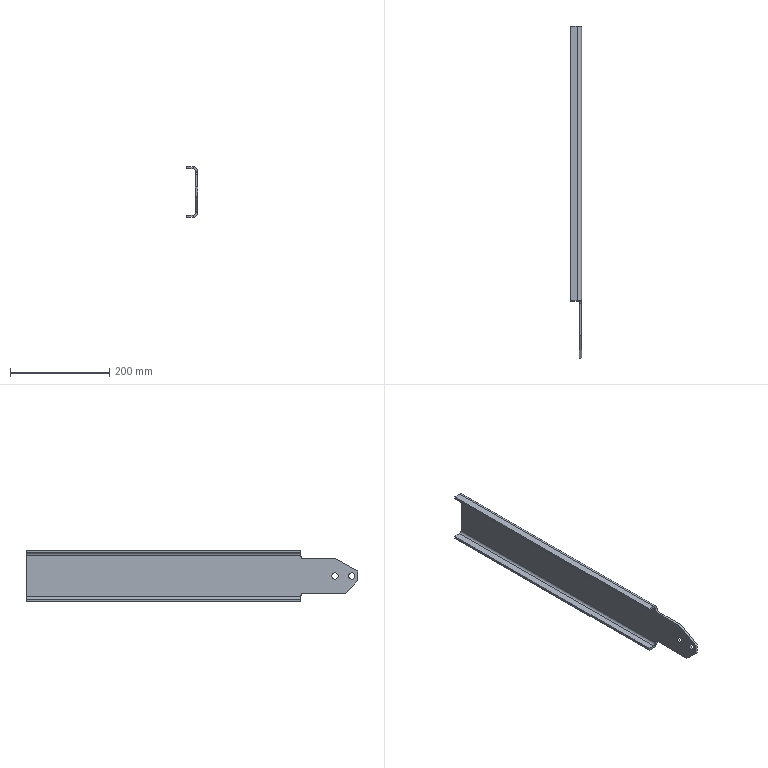Part | SolidWorks | features ICE 2, FlatPattern 1, SMBaseFlange 1, SheetMetal 1 | 1 solid | 41 faces | box 22.5 x 670 x 102.2 mm | volume 361914 mm3 | plane 26 | cylinder 15 | commonest cylinder face diameters 26.5 x5 12.5 x4 9 x2 10 x2 18 x2
STEP:
#1=CARTESIAN_POINT('',(22.499,46.5,59.85));
#2=VERTEX_POINT('',#1);
#3=CARTESIAN_POINT('',(22.499,46.5,33.35));
#4=VERTEX_POINT('',#3);
#5=CARTESIAN_POINT('',(22.499,46.5,46.6));
#6=DIRECTION('',(1.,0.,0.));
#7=DIRECTION('',(0.,0.,-1.));
#8=AXIS2_PLACEMENT_3D('',#5,#6,#7);
#9=CIRCLE('',#8,13.25);
#10=EDGE_CURVE('',#2,#4,#9,.T.);
#11=ORIENTED_EDGE('',*,*,#10,.F.);
#12=CARTESIAN_POINT('',(22.5,46.5,59.85));
#13=VERTEX_POINT('',#12);
#14=CARTESIAN_POINT('',(22.499,46.5,59.85));
#15=DIRECTION('',(1.,0.,0.));
#16=VECTOR('',#15,1000.);
#17=LINE('',#14,#16);
#18=EDGE_CURVE('',#2,#13,#17,.T.);
#19=ORIENTED_EDGE('',*,*,#18,.T.);
#20=CARTESIAN_POINT('',(22.5,46.5,33.35));
#21=VERTEX_POINT('',#20);
#22=CARTESIAN_POINT('',(22.5,46.5,46.6));
#23=DIRECTION('',(1.,0.,0.));
#24=DIRECTION('',(0.,0.,-1.));
#25=AXIS2_PLACEMENT_3D('',#22,#23,#24);
#26=CIRCLE('',#25,13.25);
#27=EDGE_CURVE('',#13,#21,#26,.T.);
#28=ORIENTED_EDGE('',*,*,#27,.T.);
#29=CARTESIAN_POINT('',(22.499,46.5,33.35));
#30=DIRECTION('',(1.,0.,0.));
#31=VECTOR('',#30,1000.);
#32=LINE('',#29,#31);
#33=EDGE_CURVE('',#4,#21,#32,.T.);
#34=ORIENTED_EDGE('',*,*,#33,.F.);
#35=EDGE_LOOP('',(#11,#19,#28,#34));
#36=FACE_OUTER_BOUND('',#35,.T.);
#37=CARTESIAN_POINT('',(22.499,46.5,46.6));
#38=DIRECTION('',(1.,0.,0.));
#39=DIRECTION('',(0.,0.,-1.));
#40=AXIS2_PLACEMENT_3D('',#37,#38,#39);
#41=CYLINDRICAL_SURFACE('',#40,13.25);
#42=ADVANCED_FACE('',(#36),#41,.F.);
#43=CARTESIAN_POINT('',(22.499,12.5,59.85));
#44=VERTEX_POINT('',#43);
#45=CARTESIAN_POINT('',(22.499,0.,50.995));
#46=VERTEX_POINT('',#45);
#47=CARTESIAN_POINT('',(22.499,12.5,46.6));
#48=DIRECTION('',(1.,0.,0.));
#49=DIRECTION('',(0.,0.,-1.));
#50=AXIS2_PLACEMENT_3D('',#47,#48,#49);
#51=CIRCLE('',#50,13.25);
#52=EDGE_CURVE('',#44,#46,#51,.T.);
#53=ORIENTED_EDGE('',*,*,#52,.F.);
#54=CARTESIAN_POINT('',(22.5,12.5,59.85));
#55=VERTEX_POINT('',#54);
#56=CARTESIAN_POINT('',(22.499,12.5,59.85));
#57=DIRECTION('',(1.,0.,0.));
#58=VECTOR('',#57,1000.);
#59=LINE('',#56,#58);
#60=EDGE_CURVE('',#44,#55,#59,.T.);
#61=ORIENTED_EDGE('',*,*,#60,.T.);
#62=CARTESIAN_POINT('',(22.5,0.,50.995));
#63=VERTEX_POINT('',#62);
#64=CARTESIAN_POINT('',(22.5,12.5,46.6));
#65=DIRECTION('',(1.,0.,0.));
#66=DIRECTION('',(0.,0.,-1.));
#67=AXIS2_PLACEMENT_3D('',#64,#65,#66);
#68=CIRCLE('',#67,13.25);
#69=EDGE_CURVE('',#55,#63,#68,.T.);
#70=ORIENTED_EDGE('',*,*,#69,.T.);
#71=CARTESIAN_POINT('',(22.499,0.,50.995));
#72=DIRECTION('',(-1.,0.,0.));
#73=VECTOR('',#72,1000.);
#74=LINE('',#71,#73);
#75=EDGE_CURVE('',#63,#46,#74,.T.);
#76=ORIENTED_EDGE('',*,*,#75,.T.);
#77=EDGE_LOOP('',(#53,#61,#70,#76));
#78=FACE_OUTER_BOUND('',#77,.T.);
#79=CARTESIAN_POINT('',(22.499,12.5,46.6));
#80=DIRECTION('',(1.,0.,0.));
#81=DIRECTION('',(0.,0.,-1.));
#82=AXIS2_PLACEMENT_3D('',#79,#80,#81);
#83=CYLINDRICAL_SURFACE('',#82,13.25);
#84=ADVANCED_FACE('',(#78),#83,.F.);
#85=ORIENTED_EDGE('',*,*,#60,.F.);
#86=CARTESIAN_POINT('',(22.499,12.5,33.35));
#87=VERTEX_POINT('',#86);
#88=CARTESIAN_POINT('',(22.499,12.5,46.6));
#89=DIRECTION('',(1.,0.,0.));
#90=DIRECTION('',(0.,0.,-1.));
#91=AXIS2_PLACEMENT_3D('',#88,#89,#90);
#92=CIRCLE('',#91,13.25);
#93=EDGE_CURVE('',#87,#44,#92,.T.);
#94=ORIENTED_EDGE('',*,*,#93,.F.);
#95=CARTESIAN_POINT('',(22.5,12.5,33.35));
#96=VERTEX_POINT('',#95);
#97=CARTESIAN_POINT('',(22.499,12.5,33.35));
#98=DIRECTION('',(1.,0.,0.));
#99=VECTOR('',#98,1000.);
#100=LINE('',#97,#99);
#101=EDGE_CURVE('',#87,#96,#100,.T.);
#102=ORIENTED_EDGE('',*,*,#101,.T.);
#103=CARTESIAN_POINT('',(22.5,12.5,46.6));
#104=DIRECTION('',(1.,0.,0.));
#105=DIRECTION('',(0.,0.,-1.));
#106=AXIS2_PLACEMENT_3D('',#103,#104,#105);
#107=CIRCLE('',#106,13.25);
#108=EDGE_CURVE('',#96,#55,#107,.T.);
#109=ORIENTED_EDGE('',*,*,#108,.T.);
#110=EDGE_LOOP('',(#85,#94,#102,#109));
#111=FACE_OUTER_BOUND('',#110,.T.);
#112=CARTESIAN_POINT('',(22.499,12.5,46.6));
#113=DIRECTION('',(1.,0.,0.));
#114=DIRECTION('',(0.,0.,-1.));
#115=AXIS2_PLACEMENT_3D('',#112,#113,#114);
#116=CYLINDRICAL_SURFACE('',#115,13.25);
#117=ADVANCED_FACE('',(#111),#116,.F.);
#118=CARTESIAN_POINT('',(18.,12.5,52.85));
#119=VERTEX_POINT('',#118);
#120=CARTESIAN_POINT('',(18.,12.5,40.35));
#121=VERTEX_POINT('',#120);
#122=CARTESIAN_POINT('',(18.,12.5,46.6));
#123=DIRECTION('',(1.,0.,0.));
#124=DIRECTION('',(0.,0.,-1.));
#125=AXIS2_PLACEMENT_3D('',#122,#123,#124);
#126=CIRCLE('',#125,6.25);
#127=EDGE_CURVE('',#119,#121,#126,.T.);
#128=ORIENTED_EDGE('',*,*,#127,.F.);
#129=CARTESIAN_POINT('',(22.499,12.5,52.85));
#130=VERTEX_POINT('',#129);
#131=CARTESIAN_POINT('',(22.5,12.5,52.85));
#132=DIRECTION('',(1.,0.,0.));
#133=VECTOR('',#132,1000.);
#134=LINE('',#131,#133);
#135=EDGE_CURVE('',#119,#130,#134,.T.);
#136=ORIENTED_EDGE('',*,*,#135,.T.);
#137=CARTESIAN_POINT('',(22.499,12.5,40.35));
#138=VERTEX_POINT('',#137);
#139=CARTESIAN_POINT('',(22.499,12.5,46.6));
#140=DIRECTION('',(1.,0.,0.));
#141=DIRECTION('',(0.,0.,-1.));
#142=AXIS2_PLACEMENT_3D('',#139,#140,#141);
#143=CIRCLE('',#142,6.25);
#144=EDGE_CURVE('',#130,#138,#143,.T.);
#145=ORIENTED_EDGE('',*,*,#144,.T.);
#146=CARTESIAN_POINT('',(22.5,12.5,40.35));
#147=DIRECTION('',(1.,0.,0.));
#148=VECTOR('',#147,1000.);
#149=LINE('',#146,#148);
#150=EDGE_CURVE('',#121,#138,#149,.T.);
#151=ORIENTED_EDGE('',*,*,#150,.F.);
#152=EDGE_LOOP('',(#128,#136,#145,#151));
#153=FACE_OUTER_BOUND('',#152,.T.);
#154=CARTESIAN_POINT('',(22.5,12.5,46.6));
#155=DIRECTION('',(1.,0.,0.));
#156=DIRECTION('',(0.,0.,-1.));
#157=AXIS2_PLACEMENT_3D('',#154,#155,#156);
#158=CYLINDRICAL_SURFACE('',#157,6.25);
#159=ADVANCED_FACE('',(#153),#158,.F.);
#160=CARTESIAN_POINT('',(18.,46.5,52.85));
#161=VERTEX_POINT('',#160);
#162=CARTESIAN_POINT('',(18.,46.5,40.35));
#163=VERTEX_POINT('',#162);
#164=CARTESIAN_POINT('',(18.,46.5,46.6));
#165=DIRECTION('',(1.,0.,0.));
#166=DIRECTION('',(0.,0.,-1.));
#167=AXIS2_PLACEMENT_3D('',#164,#165,#166);
#168=CIRCLE('',#167,6.25);
#169=EDGE_CURVE('',#161,#163,#168,.T.);
#170=ORIENTED_EDGE('',*,*,#169,.F.);
#171=CARTESIAN_POINT('',(22.499,46.5,52.85));
#172=VERTEX_POINT('',#171);
#173=CARTESIAN_POINT('',(22.5,46.5,52.85));
#174=DIRECTION('',(1.,0.,0.));
#175=VECTOR('',#174,1000.);
#176=LINE('',#173,#175);
#177=EDGE_CURVE('',#161,#172,#176,.T.);
#178=ORIENTED_EDGE('',*,*,#177,.T.);
#179=CARTESIAN_POINT('',(22.499,46.5,40.35));
#180=VERTEX_POINT('',#179);
#181=CARTESIAN_POINT('',(22.499,46.5,46.6));
#182=DIRECTION('',(1.,0.,0.));
#183=DIRECTION('',(0.,0.,-1.));
#184=AXIS2_PLACEMENT_3D('',#181,#182,#183);
#185=CIRCLE('',#184,6.25);
#186=EDGE_CURVE('',#172,#180,#185,.T.);
#187=ORIENTED_EDGE('',*,*,#186,.T.);
#188=CARTESIAN_POINT('',(22.5,46.5,40.35));
#189=DIRECTION('',(1.,0.,0.));
#190=VECTOR('',#189,1000.);
#191=LINE('',#188,#190);
#192=EDGE_CURVE('',#163,#180,#191,.T.);
#193=ORIENTED_EDGE('',*,*,#192,.F.);
#194=EDGE_LOOP('',(#170,#178,#187,#193));
#195=FACE_OUTER_BOUND('',#194,.T.);
#196=CARTESIAN_POINT('',(22.5,46.5,46.6));
#197=DIRECTION('',(1.,0.,0.));
#198=DIRECTION('',(0.,0.,-1.));
#199=AXIS2_PLACEMENT_3D('',#196,#197,#198);
#200=CYLINDRICAL_SURFACE('',#199,6.25);
#201=ADVANCED_FACE('',(#195),#200,.F.);
#202=ORIENTED_EDGE('',*,*,#177,.F.);
#203=CARTESIAN_POINT('',(18.,46.5,46.6));
#204=DIRECTION('',(1.,0.,0.));
#205=DIRECTION('',(0.,0.,-1.));
#206=AXIS2_PLACEMENT_3D('',#203,#204,#205);
#207=CIRCLE('',#206,6.25);
#208=EDGE_CURVE('',#163,#161,#207,.T.);
#209=ORIENTED_EDGE('',*,*,#208,.F.);
#210=ORIENTED_EDGE('',*,*,#192,.T.);
#211=CARTESIAN_POINT('',(22.499,46.5,46.6));
#212=DIRECTION('',(1.,0.,0.));
#213=DIRECTION('',(0.,0.,-1.));
#214=AXIS2_PLACEMENT_3D('',#211,#212,#213);
#215=CIRCLE('',#214,6.25);
#216=EDGE_CURVE('',#180,#172,#215,.T.);
#217=ORIENTED_EDGE('',*,*,#216,.T.);
#218=EDGE_LOOP('',(#202,#209,#210,#217));
#219=FACE_OUTER_BOUND('',#218,.T.);
#220=CARTESIAN_POINT('',(22.5,46.5,46.6));
#221=DIRECTION('',(1.,0.,0.));
#222=DIRECTION('',(0.,0.,-1.));
#223=AXIS2_PLACEMENT_3D('',#220,#221,#222);
#224=CYLINDRICAL_SURFACE('',#223,6.25);
#225=ADVANCED_FACE('',(#219),#224,.F.);
#226=ORIENTED_EDGE('',*,*,#135,.F.);
#227=CARTESIAN_POINT('',(18.,12.5,46.6));
#228=DIRECTION('',(1.,0.,0.));
#229=DIRECTION('',(0.,0.,-1.));
#230=AXIS2_PLACEMENT_3D('',#227,#228,#229);
#231=CIRCLE('',#230,6.25);
#232=EDGE_CURVE('',#121,#119,#231,.T.);
#233=ORIENTED_EDGE('',*,*,#232,.F.);
#234=ORIENTED_EDGE('',*,*,#150,.T.);
#235=CARTESIAN_POINT('',(22.499,12.5,46.6));
#236=DIRECTION('',(1.,0.,0.));
#237=DIRECTION('',(0.,0.,-1.));
#238=AXIS2_PLACEMENT_3D('',#235,#236,#237);
#239=CIRCLE('',#238,6.25);
#240=EDGE_CURVE('',#138,#130,#239,.T.);
#241=ORIENTED_EDGE('',*,*,#240,.T.);
#242=EDGE_LOOP('',(#226,#233,#234,#241));
#243=FACE_OUTER_BOUND('',#242,.T.);
#244=CARTESIAN_POINT('',(22.5,12.5,46.6));
#245=DIRECTION('',(1.,0.,0.));
#246=DIRECTION('',(0.,0.,-1.));
#247=AXIS2_PLACEMENT_3D('',#244,#245,#246);
#248=CYLINDRICAL_SURFACE('',#247,6.25);
#249=ADVANCED_FACE('',(#243),#248,.F.);
#250=CARTESIAN_POINT('',(22.499,0.,42.205));
#251=VERTEX_POINT('',#250);
#252=CARTESIAN_POINT('',(22.5,0.,42.205));
#253=VERTEX_POINT('',#252);
#254=CARTESIAN_POINT('',(22.499,0.,42.205));
#255=DIRECTION('',(1.,0.,0.));
#256=VECTOR('',#255,1000.);
#257=LINE('',#254,#256);
#258=EDGE_CURVE('',#251,#253,#257,.T.);
#259=ORIENTED_EDGE('',*,*,#258,.F.);
#260=CARTESIAN_POINT('',(22.499,0.,-4.5));
#261=DIRECTION('',(0.,0.,1.));
#262=VECTOR('',#261,1000.);
#263=LINE('',#260,#262);
#264=EDGE_CURVE('',#251,#46,#263,.T.);
#265=ORIENTED_EDGE('',*,*,#264,.T.);
#266=ORIENTED_EDGE('',*,*,#75,.F.);
#267=CARTESIAN_POINT('',(22.5,0.,56.7));
#268=VERTEX_POINT('',#267);
#269=CARTESIAN_POINT('',(22.5,0.,0.));
#270=DIRECTION('',(0.,0.,1.));
#271=VECTOR('',#270,1000.);
#272=LINE('',#269,#271);
#273=EDGE_CURVE('',#63,#268,#272,.T.);
#274=ORIENTED_EDGE('',*,*,#273,.T.);
#275=CARTESIAN_POINT('',(18.,0.,56.7));
#276=VERTEX_POINT('',#275);
#277=CARTESIAN_POINT('',(22.5,0.,56.7));
#278=DIRECTION('',(-1.,0.,0.));
#279=VECTOR('',#278,1000.);
#280=LINE('',#277,#279);
#281=EDGE_CURVE('',#268,#276,#280,.T.);
#282=ORIENTED_EDGE('',*,*,#281,.T.);
#283=CARTESIAN_POINT('',(18.,0.,36.7));
#284=VERTEX_POINT('',#283);
#285=CARTESIAN_POINT('',(18.,0.,0.));
#286=DIRECTION('',(0.,0.,1.));
#287=VECTOR('',#286,1000.);
#288=LINE('',#285,#287);
#289=EDGE_CURVE('',#284,#276,#288,.T.);
#290=ORIENTED_EDGE('',*,*,#289,.F.);
#291=CARTESIAN_POINT('',(22.5,0.,36.7));
#292=VERTEX_POINT('',#291);
#293=CARTESIAN_POINT('',(22.5,0.,36.7));
#294=DIRECTION('',(-1.,0.,0.));
#295=VECTOR('',#294,1000.);
#296=LINE('',#293,#295);
#297=EDGE_CURVE('',#292,#284,#296,.T.);
#298=ORIENTED_EDGE('',*,*,#297,.F.);
#299=CARTESIAN_POINT('',(22.5,0.,0.));
#300=DIRECTION('',(0.,0.,1.));
#301=VECTOR('',#300,1000.);
#302=LINE('',#299,#301);
#303=EDGE_CURVE('',#292,#253,#302,.T.);
#304=ORIENTED_EDGE('',*,*,#303,.T.);
#305=EDGE_LOOP('',(#259,#265,#266,#274,#282,#290,#298,#304));
#306=FACE_OUTER_BOUND('',#305,.T.);
#307=CARTESIAN_POINT('',(13.5,0.,-4.5));
#308=DIRECTION('',(0.,-1.,0.));
#309=DIRECTION('',(0.,0.,-1.));
#310=AXIS2_PLACEMENT_3D('',#307,#308,#309);
#311=PLANE('',#310);
#312=ADVANCED_FACE('',(#306),#311,.T.);
#313=CARTESIAN_POINT('',(0.,115.,93.2));
#314=VERTEX_POINT('',#313);
#315=CARTESIAN_POINT('',(13.5,115.,93.2));
#316=VERTEX_POINT('',#315);
#317=CARTESIAN_POINT('',(18.,115.,93.2));
#318=DIRECTION('',(1.,0.,0.));
#319=VECTOR('',#318,1000.);
#320=LINE('',#317,#319);
#321=EDGE_CURVE('',#314,#316,#320,.T.);
#322=ORIENTED_EDGE('',*,*,#321,.F.);
#323=CARTESIAN_POINT('',(0.,670.,93.2));
#324=VERTEX_POINT('',#323);
#325=CARTESIAN_POINT('',(0.,670.,93.2));
#326=DIRECTION('',(0.,-1.,0.));
#327=VECTOR('',#326,1000.);
#328=LINE('',#325,#327);
#329=EDGE_CURVE('',#324,#314,#328,.T.);
#330=ORIENTED_EDGE('',*,*,#329,.F.);
#331=CARTESIAN_POINT('',(13.5,670.,93.2));
#332=VERTEX_POINT('',#331);
#333=CARTESIAN_POINT('',(18.,670.,93.2));
#334=DIRECTION('',(-1.,0.,0.));
#335=VECTOR('',#334,1000.);
#336=LINE('',#333,#335);
#337=EDGE_CURVE('',#332,#324,#336,.T.);
#338=ORIENTED_EDGE('',*,*,#337,.F.);
#339=CARTESIAN_POINT('',(13.5,670.,93.2));
#340=DIRECTION('',(0.,-1.,0.));
#341=VECTOR('',#340,1000.);
#342=LINE('',#339,#341);
#343=EDGE_CURVE('',#332,#316,#342,.T.);
#344=ORIENTED_EDGE('',*,*,#343,.T.);
#345=EDGE_LOOP('',(#322,#330,#338,#344));
#346=FACE_OUTER_BOUND('',#345,.T.);
#347=CARTESIAN_POINT('',(18.,670.,93.2));
#348=DIRECTION('',(0.,0.,1.));
#349=DIRECTION('',(1.,0.,0.));
#350=AXIS2_PLACEMENT_3D('',#347,#348,#349);
#351=PLANE('',#350);
#352=ADVANCED_FACE('',(#346),#351,.F.);
#353=ORIENTED_EDGE('',*,*,#329,.T.);
#354=CARTESIAN_POINT('',(0.,115.,97.7));
#355=VERTEX_POINT('',#354);
#356=CARTESIAN_POINT('',(0.,115.,97.7));
#357=DIRECTION('',(0.,0.,-1.));
#358=VECTOR('',#357,1000.);
#359=LINE('',#356,#358);
#360=EDGE_CURVE('',#355,#314,#359,.T.);
#361=ORIENTED_EDGE('',*,*,#360,.F.);
#362=CARTESIAN_POINT('',(0.,670.,97.7));
#363=VERTEX_POINT('',#362);
#364=CARTESIAN_POINT('',(0.,670.,97.7));
#365=DIRECTION('',(0.,-1.,0.));
#366=VECTOR('',#365,1000.);
#367=LINE('',#364,#366);
#368=EDGE_CURVE('',#363,#355,#367,.T.);
#369=ORIENTED_EDGE('',*,*,#368,.F.);
#370=CARTESIAN_POINT('',(0.,670.,97.7));
#371=DIRECTION('',(0.,0.,-1.));
#372=VECTOR('',#371,1000.);
#373=LINE('',#370,#372);
#374=EDGE_CURVE('',#363,#324,#373,.T.);
#375=ORIENTED_EDGE('',*,*,#374,.T.);
#376=EDGE_LOOP('',(#353,#361,#369,#375));
#377=FACE_OUTER_BOUND('',#376,.T.);
#378=CARTESIAN_POINT('',(0.,670.,97.7));
#379=DIRECTION('',(-1.,0.,0.));
#380=DIRECTION('',(0.,0.,1.));
#381=AXIS2_PLACEMENT_3D('',#378,#379,#380);
#382=PLANE('',#381);
#383=ADVANCED_FACE('',(#377),#382,.T.);
#384=ORIENTED_EDGE('',*,*,#368,.T.);
#385=CARTESIAN_POINT('',(13.5,115.,97.7));
#386=VERTEX_POINT('',#385);
#387=CARTESIAN_POINT('',(-0.001,115.,97.7));
#388=DIRECTION('',(1.,0.,0.));
#389=VECTOR('',#388,1000.);
#390=LINE('',#387,#389);
#391=EDGE_CURVE('',#355,#386,#390,.T.);
#392=ORIENTED_EDGE('',*,*,#391,.T.);
#393=CARTESIAN_POINT('',(13.5,670.,97.7));
#394=VERTEX_POINT('',#393);
#395=CARTESIAN_POINT('',(13.5,670.,97.7));
#396=DIRECTION('',(0.,-1.,0.));
#397=VECTOR('',#396,1000.);
#398=LINE('',#395,#397);
#399=EDGE_CURVE('',#394,#386,#398,.T.);
#400=ORIENTED_EDGE('',*,*,#399,.F.);
#401=CARTESIAN_POINT('',(18.,670.,97.7));
#402=DIRECTION('',(-1.,0.,0.));
#403=VECTOR('',#402,1000.);
#404=LINE('',#401,#403);
#405=EDGE_CURVE('',#394,#363,#404,.T.);
#406=ORIENTED_EDGE('',*,*,#405,.T.);
#407=EDGE_LOOP('',(#384,#392,#400,#406));
#408=FACE_OUTER_BOUND('',#407,.T.);
#409=CARTESIAN_POINT('',(18.,670.,97.7));
#410=DIRECTION('',(0.,0.,1.));
#411=DIRECTION('',(1.,0.,0.));
#412=AXIS2_PLACEMENT_3D('',#409,#410,#411);
#413=PLANE('',#412);
#414=ADVANCED_FACE('',(#408),#413,.T.);
#415=ORIENTED_EDGE('',*,*,#399,.T.);
#416=CARTESIAN_POINT('',(22.5,115.,88.7));
#417=VERTEX_POINT('',#416);
#418=CARTESIAN_POINT('',(13.5,115.,88.7));
#419=DIRECTION('',(0.,1.,0.));
#420=DIRECTION('',(0.,0.,1.));
#421=AXIS2_PLACEMENT_3D('',#418,#419,#420);
#422=CIRCLE('',#421,9.);
#423=EDGE_CURVE('',#386,#417,#422,.T.);
#424=ORIENTED_EDGE('',*,*,#423,.T.);
#425=CARTESIAN_POINT('',(22.5,670.,88.7));
#426=VERTEX_POINT('',#425);
#427=CARTESIAN_POINT('',(22.5,670.,88.7));
#428=DIRECTION('',(0.,-1.,0.));
#429=VECTOR('',#428,1000.);
#430=LINE('',#427,#429);
#431=EDGE_CURVE('',#426,#417,#430,.T.);
#432=ORIENTED_EDGE('',*,*,#431,.F.);
#433=CARTESIAN_POINT('',(13.5,670.,88.7));
#434=DIRECTION('',(0.,-1.,0.));
#435=DIRECTION('',(1.,0.,0.));
#436=AXIS2_PLACEMENT_3D('',#433,#434,#435);
#437=CIRCLE('',#436,9.);
#438=EDGE_CURVE('',#426,#394,#437,.T.);
#439=ORIENTED_EDGE('',*,*,#438,.T.);
#440=EDGE_LOOP('',(#415,#424,#432,#439));
#441=FACE_OUTER_BOUND('',#440,.T.);
#442=CARTESIAN_POINT('',(13.5,670.,88.7));
#443=DIRECTION('',(0.,-1.,0.));
#444=DIRECTION('',(0.,0.,-1.));
#445=AXIS2_PLACEMENT_3D('',#442,#443,#444);
#446=CYLINDRICAL_SURFACE('',#445,9.);
#447=ADVANCED_FACE('',(#441),#446,.T.);
#448=CARTESIAN_POINT('',(22.5,670.,4.5));
#449=VERTEX_POINT('',#448);
#450=CARTESIAN_POINT('',(22.5,115.,4.5));
#451=VERTEX_POINT('',#450);
#452=CARTESIAN_POINT('',(22.5,670.,4.5));
#453=DIRECTION('',(0.,-1.,0.));
#454=VECTOR('',#453,1000.);
#455=LINE('',#452,#454);
#456=EDGE_CURVE('',#449,#451,#455,.T.);
#457=ORIENTED_EDGE('',*,*,#456,.T.);
#458=CARTESIAN_POINT('',(13.5,115.,-4.5));
#459=VERTEX_POINT('',#458);
#460=CARTESIAN_POINT('',(13.5,115.,4.5));
#461=DIRECTION('',(0.,1.,0.));
#462=DIRECTION('',(0.,0.,1.));
#463=AXIS2_PLACEMENT_3D('',#460,#461,#462);
#464=CIRCLE('',#463,9.);
#465=EDGE_CURVE('',#451,#459,#464,.T.);
#466=ORIENTED_EDGE('',*,*,#465,.T.);
#467=CARTESIAN_POINT('',(13.5,670.,-4.5));
#468=VERTEX_POINT('',#467);
#469=CARTESIAN_POINT('',(13.5,670.,-4.5));
#470=DIRECTION('',(0.,-1.,0.));
#471=VECTOR('',#470,1000.);
#472=LINE('',#469,#471);
#473=EDGE_CURVE('',#468,#459,#472,.T.);
#474=ORIENTED_EDGE('',*,*,#473,.F.);
#475=CARTESIAN_POINT('',(13.5,670.,4.5));
#476=DIRECTION('',(0.,-1.,0.));
#477=DIRECTION('',(1.,0.,0.));
#478=AXIS2_PLACEMENT_3D('',#475,#476,#477);
#479=CIRCLE('',#478,9.);
#480=EDGE_CURVE('',#468,#449,#479,.T.);
#481=ORIENTED_EDGE('',*,*,#480,.T.);
#482=EDGE_LOOP('',(#457,#466,#474,#481));
#483=FACE_OUTER_BOUND('',#482,.T.);
#484=CARTESIAN_POINT('',(13.5,670.,4.5));
#485=DIRECTION('',(0.,-1.,0.));
#486=DIRECTION('',(0.,0.,-1.));
#487=AXIS2_PLACEMENT_3D('',#484,#485,#486);
#488=CYLINDRICAL_SURFACE('',#487,9.);
#489=ADVANCED_FACE('',(#483),#488,.T.);
#490=ORIENTED_EDGE('',*,*,#473,.T.);
#491=CARTESIAN_POINT('',(0.,115.,-4.5));
#492=VERTEX_POINT('',#491);
#493=CARTESIAN_POINT('',(-0.001,115.,-4.5));
#494=DIRECTION('',(1.,0.,0.));
#495=VECTOR('',#494,1000.);
#496=LINE('',#493,#495);
#497=EDGE_CURVE('',#492,#459,#496,.T.);
#498=ORIENTED_EDGE('',*,*,#497,.F.);
#499=CARTESIAN_POINT('',(0.,670.,-4.5));
#500=VERTEX_POINT('',#499);
#501=CARTESIAN_POINT('',(0.,670.,-4.5));
#502=DIRECTION('',(0.,-1.,0.));
#503=VECTOR('',#502,1000.);
#504=LINE('',#501,#503);
#505=EDGE_CURVE('',#500,#492,#504,.T.);
#506=ORIENTED_EDGE('',*,*,#505,.F.);
#507=CARTESIAN_POINT('',(0.,670.,-4.5));
#508=DIRECTION('',(1.,0.,0.));
#509=VECTOR('',#508,1000.);
#510=LINE('',#507,#509);
#511=EDGE_CURVE('',#500,#468,#510,.T.);
#512=ORIENTED_EDGE('',*,*,#511,.T.);
#513=EDGE_LOOP('',(#490,#498,#506,#512));
#514=FACE_OUTER_BOUND('',#513,.T.);
#515=CARTESIAN_POINT('',(0.,670.,-4.5));
#516=DIRECTION('',(0.,0.,-1.));
#517=DIRECTION('',(-1.,0.,0.));
#518=AXIS2_PLACEMENT_3D('',#515,#516,#517);
#519=PLANE('',#518);
#520=ADVANCED_FACE('',(#514),#519,.T.);
#521=ORIENTED_EDGE('',*,*,#505,.T.);
#522=CARTESIAN_POINT('',(0.,115.,0.));
#523=VERTEX_POINT('',#522);
#524=CARTESIAN_POINT('',(0.,115.,-4.5));
#525=DIRECTION('',(0.,0.,1.));
#526=VECTOR('',#525,1000.);
#527=LINE('',#524,#526);
#528=EDGE_CURVE('',#492,#523,#527,.T.);
#529=ORIENTED_EDGE('',*,*,#528,.T.);
#530=CARTESIAN_POINT('',(0.,670.,0.));
#531=VERTEX_POINT('',#530);
#532=CARTESIAN_POINT('',(0.,670.,0.));
#533=DIRECTION('',(0.,-1.,0.));
#534=VECTOR('',#533,1000.);
#535=LINE('',#532,#534);
#536=EDGE_CURVE('',#531,#523,#535,.T.);
#537=ORIENTED_EDGE('',*,*,#536,.F.);
#538=CARTESIAN_POINT('',(0.,670.,0.));
#539=DIRECTION('',(0.,0.,-1.));
#540=VECTOR('',#539,1000.);
#541=LINE('',#538,#540);
#542=EDGE_CURVE('',#531,#500,#541,.T.);
#543=ORIENTED_EDGE('',*,*,#542,.T.);
#544=EDGE_LOOP('',(#521,#529,#537,#543));
#545=FACE_OUTER_BOUND('',#544,.T.);
#546=CARTESIAN_POINT('',(0.,670.,0.));
#547=DIRECTION('',(-1.,0.,0.));
#548=DIRECTION('',(0.,0.,1.));
#549=AXIS2_PLACEMENT_3D('',#546,#547,#548);
#550=PLANE('',#549);
#551=ADVANCED_FACE('',(#545),#550,.T.);
#552=CARTESIAN_POINT('',(13.5,115.,0.));
#553=VERTEX_POINT('',#552);
#554=CARTESIAN_POINT('',(0.,115.,0.));
#555=DIRECTION('',(1.,0.,0.));
#556=VECTOR('',#555,1000.);
#557=LINE('',#554,#556);
#558=EDGE_CURVE('',#523,#553,#557,.T.);
#559=ORIENTED_EDGE('',*,*,#558,.T.);
#560=CARTESIAN_POINT('',(13.5,670.,0.));
#561=VERTEX_POINT('',#560);
#562=CARTESIAN_POINT('',(13.5,670.,0.));
#563=DIRECTION('',(0.,-1.,0.));
#564=VECTOR('',#563,1000.);
#565=LINE('',#562,#564);
#566=EDGE_CURVE('',#561,#553,#565,.T.);
#567=ORIENTED_EDGE('',*,*,#566,.F.);
#568=CARTESIAN_POINT('',(0.,670.,0.));
#569=DIRECTION('',(1.,0.,0.));
#570=VECTOR('',#569,1000.);
#571=LINE('',#568,#570);
#572=EDGE_CURVE('',#531,#561,#571,.T.);
#573=ORIENTED_EDGE('',*,*,#572,.F.);
#574=ORIENTED_EDGE('',*,*,#536,.T.);
#575=EDGE_LOOP('',(#559,#567,#573,#574));
#576=FACE_OUTER_BOUND('',#575,.T.);
#577=CARTESIAN_POINT('',(0.,670.,0.));
#578=DIRECTION('',(0.,0.,-1.));
#579=DIRECTION('',(-1.,0.,0.));
#580=AXIS2_PLACEMENT_3D('',#577,#578,#579);
#581=PLANE('',#580);
#582=ADVANCED_FACE('',(#576),#581,.F.);
#583=CARTESIAN_POINT('',(18.,115.,4.5));
#584=VERTEX_POINT('',#583);
#585=CARTESIAN_POINT('',(13.5,115.,4.5));
#586=DIRECTION('',(0.,1.,0.));
#587=DIRECTION('',(0.,0.,-1.));
#588=AXIS2_PLACEMENT_3D('',#585,#586,#587);
#589=CIRCLE('',#588,4.5);
#590=EDGE_CURVE('',#584,#553,#589,.T.);
#591=ORIENTED_EDGE('',*,*,#590,.F.);
#592=CARTESIAN_POINT('',(18.,670.,4.5));
#593=VERTEX_POINT('',#592);
#594=CARTESIAN_POINT('',(18.,670.,4.5));
#595=DIRECTION('',(0.,-1.,0.));
#596=VECTOR('',#595,1000.);
#597=LINE('',#594,#596);
#598=EDGE_CURVE('',#593,#584,#597,.T.);
#599=ORIENTED_EDGE('',*,*,#598,.F.);
#600=CARTESIAN_POINT('',(13.5,670.,4.5));
#601=DIRECTION('',(0.,-1.,0.));
#602=DIRECTION('',(0.,0.,1.));
#603=AXIS2_PLACEMENT_3D('',#600,#601,#602);
#604=CIRCLE('',#603,4.5);
#605=EDGE_CURVE('',#561,#593,#604,.T.);
#606=ORIENTED_EDGE('',*,*,#605,.F.);
#607=ORIENTED_EDGE('',*,*,#566,.T.);
#608=EDGE_LOOP('',(#591,#599,#606,#607));
#609=FACE_OUTER_BOUND('',#608,.T.);
#610=CARTESIAN_POINT('',(13.5,670.,4.5));
#611=DIRECTION('',(0.,-1.,0.));
#612=DIRECTION('',(0.,0.,-1.));
#613=AXIS2_PLACEMENT_3D('',#610,#611,#612);
#614=CYLINDRICAL_SURFACE('',#613,4.5);
#615=ADVANCED_FACE('',(#609),#614,.F.);
#616=CARTESIAN_POINT('',(18.,115.,88.7));
#617=VERTEX_POINT('',#616);
#618=CARTESIAN_POINT('',(13.5,115.,88.7));
#619=DIRECTION('',(0.,1.,0.));
#620=DIRECTION('',(0.,0.,-1.));
#621=AXIS2_PLACEMENT_3D('',#618,#619,#620);
#622=CIRCLE('',#621,4.5);
#623=EDGE_CURVE('',#316,#617,#622,.T.);
#624=ORIENTED_EDGE('',*,*,#623,.F.);
#625=ORIENTED_EDGE('',*,*,#343,.F.);
#626=CARTESIAN_POINT('',(18.,670.,88.7));
#627=VERTEX_POINT('',#626);
#628=CARTESIAN_POINT('',(13.5,670.,88.7));
#629=DIRECTION('',(0.,-1.,0.));
#630=DIRECTION('',(0.,0.,1.));
#631=AXIS2_PLACEMENT_3D('',#628,#629,#630);
#632=CIRCLE('',#631,4.5);
#633=EDGE_CURVE('',#627,#332,#632,.T.);
#634=ORIENTED_EDGE('',*,*,#633,.F.);
#635=CARTESIAN_POINT('',(18.,670.,88.7));
#636=DIRECTION('',(0.,-1.,0.));
#637=VECTOR('',#636,1000.);
#638=LINE('',#635,#637);
#639=EDGE_CURVE('',#627,#617,#638,.T.);
#640=ORIENTED_EDGE('',*,*,#639,.T.);
#641=EDGE_LOOP('',(#624,#625,#634,#640));
#642=FACE_OUTER_BOUND('',#641,.T.);
#643=CARTESIAN_POINT('',(13.5,670.,88.7));
#644=DIRECTION('',(0.,-1.,0.));
#645=DIRECTION('',(0.,0.,-1.));
#646=AXIS2_PLACEMENT_3D('',#643,#644,#645);
#647=CYLINDRICAL_SURFACE('',#646,4.5);
#648=ADVANCED_FACE('',(#642),#647,.F.);
#649=CARTESIAN_POINT('',(13.5,670.,0.));
#650=DIRECTION('',(0.,0.,-1.));
#651=VECTOR('',#650,1000.);
#652=LINE('',#649,#651);
#653=EDGE_CURVE('',#561,#468,#652,.T.);
#654=ORIENTED_EDGE('',*,*,#653,.F.);
#655=ORIENTED_EDGE('',*,*,#605,.T.);
#656=CARTESIAN_POINT('',(22.5,670.,4.5));
#657=DIRECTION('',(-1.,0.,0.));
#658=VECTOR('',#657,1000.);
#659=LINE('',#656,#658);
#660=EDGE_CURVE('',#449,#593,#659,.T.);
#661=ORIENTED_EDGE('',*,*,#660,.F.);
#662=ORIENTED_EDGE('',*,*,#480,.F.);
#663=EDGE_LOOP('',(#654,#655,#661,#662));
#664=FACE_OUTER_BOUND('',#663,.T.);
#665=CARTESIAN_POINT('',(13.5,670.,0.));
#666=DIRECTION('',(0.,1.,0.));
#667=DIRECTION('',(0.,0.,1.));
#668=AXIS2_PLACEMENT_3D('',#665,#666,#667);
#669=PLANE('',#668);
#670=ADVANCED_FACE('',(#664),#669,.T.);
#671=ORIENTED_EDGE('',*,*,#572,.T.);
#672=ORIENTED_EDGE('',*,*,#653,.T.);
#673=ORIENTED_EDGE('',*,*,#511,.F.);
#674=ORIENTED_EDGE('',*,*,#542,.F.);
#675=EDGE_LOOP('',(#671,#672,#673,#674));
#676=FACE_OUTER_BOUND('',#675,.T.);
#677=CARTESIAN_POINT('',(22.5,670.,4.5));
#678=DIRECTION('',(0.,1.,0.));
#679=DIRECTION('',(0.,0.,1.));
#680=AXIS2_PLACEMENT_3D('',#677,#678,#679);
#681=PLANE('',#680);
#682=ADVANCED_FACE('',(#676),#681,.T.);
#683=CARTESIAN_POINT('',(18.,670.,88.7));
#684=DIRECTION('',(1.,0.,0.));
#685=VECTOR('',#684,1000.);
#686=LINE('',#683,#685);
#687=EDGE_CURVE('',#627,#426,#686,.T.);
#688=ORIENTED_EDGE('',*,*,#687,.F.);
#689=ORIENTED_EDGE('',*,*,#633,.T.);
#690=CARTESIAN_POINT('',(13.5,670.,97.7));
#691=DIRECTION('',(0.,0.,-1.));
#692=VECTOR('',#691,1000.);
#693=LINE('',#690,#692);
#694=EDGE_CURVE('',#394,#332,#693,.T.);
#695=ORIENTED_EDGE('',*,*,#694,.F.);
#696=ORIENTED_EDGE('',*,*,#438,.F.);
#697=EDGE_LOOP('',(#688,#689,#695,#696));
#698=FACE_OUTER_BOUND('',#697,.T.);
#699=CARTESIAN_POINT('',(18.,670.,88.7));
#700=DIRECTION('',(0.,1.,0.));
#701=DIRECTION('',(0.,0.,1.));
#702=AXIS2_PLACEMENT_3D('',#699,#700,#701);
#703=PLANE('',#702);
#704=ADVANCED_FACE('',(#698),#703,.T.);
#705=CARTESIAN_POINT('',(18.,670.,0.));
#706=DIRECTION('',(0.,0.,1.));
#707=VECTOR('',#706,1000.);
#708=LINE('',#705,#707);
#709=EDGE_CURVE('',#593,#627,#708,.T.);
#710=ORIENTED_EDGE('',*,*,#709,.T.);
#711=ORIENTED_EDGE('',*,*,#687,.T.);
#712=CARTESIAN_POINT('',(22.5,670.,0.));
#713=DIRECTION('',(0.,0.,1.));
#714=VECTOR('',#713,1000.);
#715=LINE('',#712,#714);
#716=EDGE_CURVE('',#449,#426,#715,.T.);
#717=ORIENTED_EDGE('',*,*,#716,.F.);
#718=ORIENTED_EDGE('',*,*,#660,.T.);
#719=EDGE_LOOP('',(#710,#711,#717,#718));
#720=FACE_OUTER_BOUND('',#719,.T.);
#721=CARTESIAN_POINT('',(13.5,670.,97.7));
#722=DIRECTION('',(0.,1.,0.));
#723=DIRECTION('',(0.,0.,1.));
#724=AXIS2_PLACEMENT_3D('',#721,#722,#723);
#725=PLANE('',#724);
#726=ADVANCED_FACE('',(#720),#725,.T.);
#727=CARTESIAN_POINT('',(22.5,46.5,46.6));
#728=DIRECTION('',(1.,0.,0.));
#729=DIRECTION('',(0.,0.,-1.));
#730=AXIS2_PLACEMENT_3D('',#727,#728,#729);
#731=CIRCLE('',#730,13.25);
#732=EDGE_CURVE('',#21,#13,#731,.T.);
#733=ORIENTED_EDGE('',*,*,#732,.F.);
#734=ORIENTED_EDGE('',*,*,#27,.F.);
#735=EDGE_LOOP('',(#733,#734));
#736=FACE_BOUND('',#735,.T.);
#737=CARTESIAN_POINT('',(22.5,12.5,46.6));
#738=DIRECTION('',(1.,0.,0.));
#739=DIRECTION('',(0.,0.,-1.));
#740=AXIS2_PLACEMENT_3D('',#737,#738,#739);
#741=CIRCLE('',#740,13.25);
#742=EDGE_CURVE('',#253,#96,#741,.T.);
#743=ORIENTED_EDGE('',*,*,#742,.F.);
#744=ORIENTED_EDGE('',*,*,#303,.F.);
#745=CARTESIAN_POINT('',(22.5,25.,11.7));
#746=VERTEX_POINT('',#745);
#747=CARTESIAN_POINT('',(22.5,0.,36.7));
#748=DIRECTION('',(0.,-0.7071,0.7071));
#749=VECTOR('',#748,1000.);
#750=LINE('',#747,#749);
#751=EDGE_CURVE('',#746,#292,#750,.T.);
#752=ORIENTED_EDGE('',*,*,#751,.F.);
#753=CARTESIAN_POINT('',(22.5,110.,11.7));
#754=VERTEX_POINT('',#753);
#755=CARTESIAN_POINT('',(22.5,25.,11.7));
#756=DIRECTION('',(0.,-1.,0.));
#757=VECTOR('',#756,1000.);
#758=LINE('',#755,#757);
#759=EDGE_CURVE('',#754,#746,#758,.T.);
#760=ORIENTED_EDGE('',*,*,#759,.F.);
#761=CARTESIAN_POINT('',(22.5,115.,6.7));
#762=VERTEX_POINT('',#761);
#763=CARTESIAN_POINT('',(22.5,110.,6.7));
#764=DIRECTION('',(1.,0.,0.));
#765=DIRECTION('',(0.,0.,1.));
#766=AXIS2_PLACEMENT_3D('',#763,#764,#765);
#767=CIRCLE('',#766,5.);
#768=EDGE_CURVE('',#762,#754,#767,.T.);
#769=ORIENTED_EDGE('',*,*,#768,.F.);
#770=CARTESIAN_POINT('',(22.5,115.,6.7));
#771=DIRECTION('',(0.,0.,1.));
#772=VECTOR('',#771,1000.);
#773=LINE('',#770,#772);
#774=EDGE_CURVE('',#451,#762,#773,.T.);
#775=ORIENTED_EDGE('',*,*,#774,.F.);
#776=ORIENTED_EDGE('',*,*,#456,.F.);
#777=ORIENTED_EDGE('',*,*,#716,.T.);
#778=ORIENTED_EDGE('',*,*,#431,.T.);
#779=CARTESIAN_POINT('',(22.5,115.,86.7));
#780=VERTEX_POINT('',#779);
#781=CARTESIAN_POINT('',(22.5,115.,86.7));
#782=DIRECTION('',(0.,0.,1.));
#783=VECTOR('',#782,1000.);
#784=LINE('',#781,#783);
#785=EDGE_CURVE('',#780,#417,#784,.T.);
#786=ORIENTED_EDGE('',*,*,#785,.F.);
#787=CARTESIAN_POINT('',(22.5,110.,81.7));
#788=VERTEX_POINT('',#787);
#789=CARTESIAN_POINT('',(22.5,110.,86.7));
#790=DIRECTION('',(1.,0.,0.));
#791=DIRECTION('',(0.,0.,-1.));
#792=AXIS2_PLACEMENT_3D('',#789,#790,#791);
#793=CIRCLE('',#792,5.);
#794=EDGE_CURVE('',#788,#780,#793,.T.);
#795=ORIENTED_EDGE('',*,*,#794,.F.);
#796=CARTESIAN_POINT('',(22.5,45.,81.7));
#797=VERTEX_POINT('',#796);
#798=CARTESIAN_POINT('',(22.5,45.,81.7));
#799=DIRECTION('',(0.,1.,0.));
#800=VECTOR('',#799,1000.);
#801=LINE('',#798,#800);
#802=EDGE_CURVE('',#797,#788,#801,.T.);
#803=ORIENTED_EDGE('',*,*,#802,.F.);
#804=CARTESIAN_POINT('',(22.5,0.,56.7));
#805=DIRECTION('',(0.,0.8742,0.4856));
#806=VECTOR('',#805,1000.);
#807=LINE('',#804,#806);
#808=EDGE_CURVE('',#268,#797,#807,.T.);
#809=ORIENTED_EDGE('',*,*,#808,.F.);
#810=ORIENTED_EDGE('',*,*,#273,.F.);
#811=ORIENTED_EDGE('',*,*,#69,.F.);
#812=ORIENTED_EDGE('',*,*,#108,.F.);
#813=EDGE_LOOP('',(#743,#744,#752,#760,#769,#775,#776,#777,#778,#786,#795,#803,#809,#810,#811,#812));
#814=FACE_OUTER_BOUND('',#813,.T.);
#815=CARTESIAN_POINT('',(22.5,670.,0.));
#816=DIRECTION('',(1.,0.,0.));
#817=DIRECTION('',(0.,0.,-1.));
#818=AXIS2_PLACEMENT_3D('',#815,#816,#817);
#819=PLANE('',#818);
#820=ADVANCED_FACE('',(#736,#814),#819,.T.);
#821=CARTESIAN_POINT('',(18.,45.,81.7));
#822=VERTEX_POINT('',#821);
#823=CARTESIAN_POINT('',(18.,0.,56.7));
#824=DIRECTION('',(0.,0.8742,0.4856));
#825=VECTOR('',#824,1000.);
#826=LINE('',#823,#825);
#827=EDGE_CURVE('',#276,#822,#826,.T.);
#828=ORIENTED_EDGE('',*,*,#827,.T.);
#829=CARTESIAN_POINT('',(18.,110.,81.7));
#830=VERTEX_POINT('',#829);
#831=CARTESIAN_POINT('',(18.,670.,81.7));
#832=DIRECTION('',(0.,1.,0.));
#833=VECTOR('',#832,1000.);
#834=LINE('',#831,#833);
#835=EDGE_CURVE('',#822,#830,#834,.T.);
#836=ORIENTED_EDGE('',*,*,#835,.T.);
#837=CARTESIAN_POINT('',(18.,115.,86.7));
#838=VERTEX_POINT('',#837);
#839=CARTESIAN_POINT('',(18.,110.,86.7));
#840=DIRECTION('',(1.,0.,0.));
#841=DIRECTION('',(0.,0.,-1.));
#842=AXIS2_PLACEMENT_3D('',#839,#840,#841);
#843=CIRCLE('',#842,5.);
#844=EDGE_CURVE('',#830,#838,#843,.T.);
#845=ORIENTED_EDGE('',*,*,#844,.T.);
#846=CARTESIAN_POINT('',(18.,115.,0.));
#847=DIRECTION('',(0.,0.,1.));
#848=VECTOR('',#847,1000.);
#849=LINE('',#846,#848);
#850=EDGE_CURVE('',#838,#617,#849,.T.);
#851=ORIENTED_EDGE('',*,*,#850,.T.);
#852=ORIENTED_EDGE('',*,*,#639,.F.);
#853=ORIENTED_EDGE('',*,*,#709,.F.);
#854=ORIENTED_EDGE('',*,*,#598,.T.);
#855=CARTESIAN_POINT('',(18.,115.,6.7));
#856=VERTEX_POINT('',#855);
#857=CARTESIAN_POINT('',(18.,115.,0.));
#858=DIRECTION('',(0.,0.,1.));
#859=VECTOR('',#858,1000.);
#860=LINE('',#857,#859);
#861=EDGE_CURVE('',#584,#856,#860,.T.);
#862=ORIENTED_EDGE('',*,*,#861,.T.);
#863=CARTESIAN_POINT('',(18.,110.,11.7));
#864=VERTEX_POINT('',#863);
#865=CARTESIAN_POINT('',(18.,110.,6.7));
#866=DIRECTION('',(1.,0.,0.));
#867=DIRECTION('',(0.,0.,-1.));
#868=AXIS2_PLACEMENT_3D('',#865,#866,#867);
#869=CIRCLE('',#868,5.);
#870=EDGE_CURVE('',#856,#864,#869,.T.);
#871=ORIENTED_EDGE('',*,*,#870,.T.);
#872=CARTESIAN_POINT('',(18.,25.,11.7));
#873=VERTEX_POINT('',#872);
#874=CARTESIAN_POINT('',(18.,670.,11.7));
#875=DIRECTION('',(0.,-1.,0.));
#876=VECTOR('',#875,1000.);
#877=LINE('',#874,#876);
#878=EDGE_CURVE('',#864,#873,#877,.T.);
#879=ORIENTED_EDGE('',*,*,#878,.T.);
#880=CARTESIAN_POINT('',(18.,0.,36.7));
#881=DIRECTION('',(0.,-0.7071,0.7071));
#882=VECTOR('',#881,1000.);
#883=LINE('',#880,#882);
#884=EDGE_CURVE('',#873,#284,#883,.T.);
#885=ORIENTED_EDGE('',*,*,#884,.T.);
#886=ORIENTED_EDGE('',*,*,#289,.T.);
#887=EDGE_LOOP('',(#828,#836,#845,#851,#852,#853,#854,#862,#871,#879,#885,#886));
#888=FACE_OUTER_BOUND('',#887,.T.);
#889=ORIENTED_EDGE('',*,*,#232,.T.);
#890=ORIENTED_EDGE('',*,*,#127,.T.);
#891=EDGE_LOOP('',(#889,#890));
#892=FACE_BOUND('',#891,.T.);
#893=ORIENTED_EDGE('',*,*,#208,.T.);
#894=ORIENTED_EDGE('',*,*,#169,.T.);
#895=EDGE_LOOP('',(#893,#894));
#896=FACE_BOUND('',#895,.T.);
#897=CARTESIAN_POINT('',(18.,670.,0.));
#898=DIRECTION('',(1.,0.,0.));
#899=DIRECTION('',(0.,0.,-1.));
#900=AXIS2_PLACEMENT_3D('',#897,#898,#899);
#901=PLANE('',#900);
#902=ADVANCED_FACE('',(#888,#892,#896),#901,.F.);
#903=ORIENTED_EDGE('',*,*,#337,.T.);
#904=ORIENTED_EDGE('',*,*,#374,.F.);
#905=ORIENTED_EDGE('',*,*,#405,.F.);
#906=ORIENTED_EDGE('',*,*,#694,.T.);
#907=EDGE_LOOP('',(#903,#904,#905,#906));
#908=FACE_OUTER_BOUND('',#907,.T.);
#909=CARTESIAN_POINT('',(13.5,670.,88.7));
#910=DIRECTION('',(0.,1.,0.));
#911=DIRECTION('',(1.,0.,0.));
#912=AXIS2_PLACEMENT_3D('',#909,#910,#911);
#913=PLANE('',#912);
#914=ADVANCED_FACE('',(#908),#913,.T.);
#915=ORIENTED_EDGE('',*,*,#281,.F.);
#916=ORIENTED_EDGE('',*,*,#808,.T.);
#917=CARTESIAN_POINT('',(22.5,45.,81.7));
#918=DIRECTION('',(-1.,0.,0.));
#919=VECTOR('',#918,1000.);
#920=LINE('',#917,#919);
#921=EDGE_CURVE('',#797,#822,#920,.T.);
#922=ORIENTED_EDGE('',*,*,#921,.T.);
#923=ORIENTED_EDGE('',*,*,#827,.F.);
#924=EDGE_LOOP('',(#915,#916,#922,#923));
#925=FACE_OUTER_BOUND('',#924,.T.);
#926=CARTESIAN_POINT('',(22.5,0.,56.7));
#927=DIRECTION('',(0.,0.4856,-0.8742));
#928=DIRECTION('',(0.,0.8742,0.4856));
#929=AXIS2_PLACEMENT_3D('',#926,#927,#928);
#930=PLANE('',#929);
#931=ADVANCED_FACE('',(#925),#930,.F.);
#932=ORIENTED_EDGE('',*,*,#921,.F.);
#933=ORIENTED_EDGE('',*,*,#802,.T.);
#934=CARTESIAN_POINT('',(22.5,110.,81.7));
#935=DIRECTION('',(-1.,0.,0.));
#936=VECTOR('',#935,1000.);
#937=LINE('',#934,#936);
#938=EDGE_CURVE('',#788,#830,#937,.T.);
#939=ORIENTED_EDGE('',*,*,#938,.T.);
#940=ORIENTED_EDGE('',*,*,#835,.F.);
#941=EDGE_LOOP('',(#932,#933,#939,#940));
#942=FACE_OUTER_BOUND('',#941,.T.);
#943=CARTESIAN_POINT('',(22.5,45.,81.7));
#944=DIRECTION('',(0.,0.,-1.));
#945=DIRECTION('',(0.,1.,0.));
#946=AXIS2_PLACEMENT_3D('',#943,#944,#945);
#947=PLANE('',#946);
#948=ADVANCED_FACE('',(#942),#947,.F.);
#949=ORIENTED_EDGE('',*,*,#938,.F.);
#950=ORIENTED_EDGE('',*,*,#794,.T.);
#951=CARTESIAN_POINT('',(22.5,115.,86.7));
#952=DIRECTION('',(-1.,0.,0.));
#953=VECTOR('',#952,1000.);
#954=LINE('',#951,#953);
#955=EDGE_CURVE('',#780,#838,#954,.T.);
#956=ORIENTED_EDGE('',*,*,#955,.T.);
#957=ORIENTED_EDGE('',*,*,#844,.F.);
#958=EDGE_LOOP('',(#949,#950,#956,#957));
#959=FACE_OUTER_BOUND('',#958,.T.);
#960=CARTESIAN_POINT('',(22.5,110.,86.7));
#961=DIRECTION('',(1.,0.,0.));
#962=DIRECTION('',(0.,0.,-1.));
#963=AXIS2_PLACEMENT_3D('',#960,#961,#962);
#964=CYLINDRICAL_SURFACE('',#963,5.);
#965=ADVANCED_FACE('',(#959),#964,.F.);
#966=ORIENTED_EDGE('',*,*,#785,.T.);
#967=CARTESIAN_POINT('',(22.5,115.,88.7));
#968=DIRECTION('',(-1.,0.,0.));
#969=VECTOR('',#968,1000.);
#970=LINE('',#967,#969);
#971=EDGE_CURVE('',#417,#617,#970,.T.);
#972=ORIENTED_EDGE('',*,*,#971,.T.);
#973=ORIENTED_EDGE('',*,*,#850,.F.);
#974=ORIENTED_EDGE('',*,*,#955,.F.);
#975=EDGE_LOOP('',(#966,#972,#973,#974));
#976=FACE_OUTER_BOUND('',#975,.T.);
#977=CARTESIAN_POINT('',(22.5,115.,86.7));
#978=DIRECTION('',(0.,1.,0.));
#979=DIRECTION('',(0.,0.,1.));
#980=AXIS2_PLACEMENT_3D('',#977,#978,#979);
#981=PLANE('',#980);
#982=ADVANCED_FACE('',(#976),#981,.F.);
#983=ORIENTED_EDGE('',*,*,#423,.F.);
#984=CARTESIAN_POINT('',(13.5,115.,97.7));
#985=DIRECTION('',(0.,0.,-1.));
#986=VECTOR('',#985,1000.);
#987=LINE('',#984,#986);
#988=EDGE_CURVE('',#386,#316,#987,.T.);
#989=ORIENTED_EDGE('',*,*,#988,.T.);
#990=ORIENTED_EDGE('',*,*,#623,.T.);
#991=ORIENTED_EDGE('',*,*,#971,.F.);
#992=EDGE_LOOP('',(#983,#989,#990,#991));
#993=FACE_OUTER_BOUND('',#992,.T.);
#994=CARTESIAN_POINT('',(13.5,115.,88.7));
#995=DIRECTION('',(0.,-1.,0.));
#996=DIRECTION('',(0.,0.,-1.));
#997=AXIS2_PLACEMENT_3D('',#994,#995,#996);
#998=PLANE('',#997);
#999=ADVANCED_FACE('',(#993),#998,.T.);
#1000=ORIENTED_EDGE('',*,*,#391,.F.);
#1001=ORIENTED_EDGE('',*,*,#360,.T.);
#1002=ORIENTED_EDGE('',*,*,#321,.T.);
#1003=ORIENTED_EDGE('',*,*,#988,.F.);
#1004=EDGE_LOOP('',(#1000,#1001,#1002,#1003));
#1005=FACE_OUTER_BOUND('',#1004,.T.);
#1006=CARTESIAN_POINT('',(-0.001,115.,97.7));
#1007=DIRECTION('',(0.,-1.,0.));
#1008=DIRECTION('',(1.,0.,0.));
#1009=AXIS2_PLACEMENT_3D('',#1006,#1007,#1008);
#1010=PLANE('',#1009);
#1011=ADVANCED_FACE('',(#1005),#1010,.T.);
#1012=CARTESIAN_POINT('',(22.5,115.,4.5));
#1013=DIRECTION('',(-1.,0.,0.));
#1014=VECTOR('',#1013,1000.);
#1015=LINE('',#1012,#1014);
#1016=EDGE_CURVE('',#451,#584,#1015,.T.);
#1017=ORIENTED_EDGE('',*,*,#1016,.F.);
#1018=ORIENTED_EDGE('',*,*,#774,.T.);
#1019=CARTESIAN_POINT('',(22.5,115.,6.7));
#1020=DIRECTION('',(-1.,0.,0.));
#1021=VECTOR('',#1020,1000.);
#1022=LINE('',#1019,#1021);
#1023=EDGE_CURVE('',#762,#856,#1022,.T.);
#1024=ORIENTED_EDGE('',*,*,#1023,.T.);
#1025=ORIENTED_EDGE('',*,*,#861,.F.);
#1026=EDGE_LOOP('',(#1017,#1018,#1024,#1025));
#1027=FACE_OUTER_BOUND('',#1026,.T.);
#1028=CARTESIAN_POINT('',(22.5,115.,6.7));
#1029=DIRECTION('',(0.,1.,0.));
#1030=DIRECTION('',(0.,0.,1.));
#1031=AXIS2_PLACEMENT_3D('',#1028,#1029,#1030);
#1032=PLANE('',#1031);
#1033=ADVANCED_FACE('',(#1027),#1032,.F.);
#1034=ORIENTED_EDGE('',*,*,#1023,.F.);
#1035=ORIENTED_EDGE('',*,*,#768,.T.);
#1036=CARTESIAN_POINT('',(22.5,110.,11.7));
#1037=DIRECTION('',(-1.,0.,0.));
#1038=VECTOR('',#1037,1000.);
#1039=LINE('',#1036,#1038);
#1040=EDGE_CURVE('',#754,#864,#1039,.T.);
#1041=ORIENTED_EDGE('',*,*,#1040,.T.);
#1042=ORIENTED_EDGE('',*,*,#870,.F.);
#1043=EDGE_LOOP('',(#1034,#1035,#1041,#1042));
#1044=FACE_OUTER_BOUND('',#1043,.T.);
#1045=CARTESIAN_POINT('',(22.5,110.,6.7));
#1046=DIRECTION('',(1.,0.,0.));
#1047=DIRECTION('',(0.,0.,-1.));
#1048=AXIS2_PLACEMENT_3D('',#1045,#1046,#1047);
#1049=CYLINDRICAL_SURFACE('',#1048,5.);
#1050=ADVANCED_FACE('',(#1044),#1049,.F.);
#1051=ORIENTED_EDGE('',*,*,#1040,.F.);
#1052=ORIENTED_EDGE('',*,*,#759,.T.);
#1053=CARTESIAN_POINT('',(22.5,25.,11.7));
#1054=DIRECTION('',(-1.,0.,0.));
#1055=VECTOR('',#1054,1000.);
#1056=LINE('',#1053,#1055);
#1057=EDGE_CURVE('',#746,#873,#1056,.T.);
#1058=ORIENTED_EDGE('',*,*,#1057,.T.);
#1059=ORIENTED_EDGE('',*,*,#878,.F.);
#1060=EDGE_LOOP('',(#1051,#1052,#1058,#1059));
#1061=FACE_OUTER_BOUND('',#1060,.T.);
#1062=CARTESIAN_POINT('',(22.5,25.,11.7));
#1063=DIRECTION('',(0.,0.,1.));
#1064=DIRECTION('',(0.,-1.,0.));
#1065=AXIS2_PLACEMENT_3D('',#1062,#1063,#1064);
#1066=PLANE('',#1065);
#1067=ADVANCED_FACE('',(#1061),#1066,.F.);
#1068=ORIENTED_EDGE('',*,*,#751,.T.);
#1069=ORIENTED_EDGE('',*,*,#297,.T.);
#1070=ORIENTED_EDGE('',*,*,#884,.F.);
#1071=ORIENTED_EDGE('',*,*,#1057,.F.);
#1072=EDGE_LOOP('',(#1068,#1069,#1070,#1071));
#1073=FACE_OUTER_BOUND('',#1072,.T.);
#1074=CARTESIAN_POINT('',(22.5,0.,36.7));
#1075=DIRECTION('',(0.,0.7071,0.7071));
#1076=DIRECTION('',(0.,-0.7071,0.7071));
#1077=AXIS2_PLACEMENT_3D('',#1074,#1075,#1076);
#1078=PLANE('',#1077);
#1079=ADVANCED_FACE('',(#1073),#1078,.F.);
#1080=ORIENTED_EDGE('',*,*,#497,.T.);
#1081=CARTESIAN_POINT('',(13.5,115.,-4.5));
#1082=DIRECTION('',(0.,0.,1.));
#1083=VECTOR('',#1082,1000.);
#1084=LINE('',#1081,#1083);
#1085=EDGE_CURVE('',#459,#553,#1084,.T.);
#1086=ORIENTED_EDGE('',*,*,#1085,.T.);
#1087=ORIENTED_EDGE('',*,*,#558,.F.);
#1088=ORIENTED_EDGE('',*,*,#528,.F.);
#1089=EDGE_LOOP('',(#1080,#1086,#1087,#1088));
#1090=FACE_OUTER_BOUND('',#1089,.T.);
#1091=CARTESIAN_POINT('',(-0.001,115.,-4.5));
#1092=DIRECTION('',(0.,1.,0.));
#1093=DIRECTION('',(1.,0.,0.));
#1094=AXIS2_PLACEMENT_3D('',#1091,#1092,#1093);
#1095=PLANE('',#1094);
#1096=ADVANCED_FACE('',(#1090),#1095,.F.);
#1097=ORIENTED_EDGE('',*,*,#465,.F.);
#1098=ORIENTED_EDGE('',*,*,#1016,.T.);
#1099=ORIENTED_EDGE('',*,*,#590,.T.);
#1100=ORIENTED_EDGE('',*,*,#1085,.F.);
#1101=EDGE_LOOP('',(#1097,#1098,#1099,#1100));
#1102=FACE_OUTER_BOUND('',#1101,.T.);
#1103=CARTESIAN_POINT('',(13.5,115.,4.5));
#1104=DIRECTION('',(0.,-1.,0.));
#1105=DIRECTION('',(0.,0.,-1.));
#1106=AXIS2_PLACEMENT_3D('',#1103,#1104,#1105);
#1107=PLANE('',#1106);
#1108=ADVANCED_FACE('',(#1102),#1107,.T.);
#1109=ORIENTED_EDGE('',*,*,#101,.F.);
#1110=CARTESIAN_POINT('',(22.499,12.5,46.6));
#1111=DIRECTION('',(1.,0.,0.));
#1112=DIRECTION('',(0.,0.,-1.));
#1113=AXIS2_PLACEMENT_3D('',#1110,#1111,#1112);
#1114=CIRCLE('',#1113,13.25);
#1115=EDGE_CURVE('',#251,#87,#1114,.T.);
#1116=ORIENTED_EDGE('',*,*,#1115,.F.);
#1117=ORIENTED_EDGE('',*,*,#258,.T.);
#1118=ORIENTED_EDGE('',*,*,#742,.T.);
#1119=EDGE_LOOP('',(#1109,#1116,#1117,#1118));
#1120=FACE_OUTER_BOUND('',#1119,.T.);
#1121=CARTESIAN_POINT('',(22.499,12.5,46.6));
#1122=DIRECTION('',(1.,0.,0.));
#1123=DIRECTION('',(0.,0.,-1.));
#1124=AXIS2_PLACEMENT_3D('',#1121,#1122,#1123);
#1125=CYLINDRICAL_SURFACE('',#1124,13.25);
#1126=ADVANCED_FACE('',(#1120),#1125,.F.);
#1127=ORIENTED_EDGE('',*,*,#240,.F.);
#1128=ORIENTED_EDGE('',*,*,#144,.F.);
#1129=EDGE_LOOP('',(#1127,#1128));
#1130=FACE_BOUND('',#1129,.T.);
#1131=ORIENTED_EDGE('',*,*,#1115,.T.);
#1132=ORIENTED_EDGE('',*,*,#93,.T.);
#1133=ORIENTED_EDGE('',*,*,#52,.T.);
#1134=ORIENTED_EDGE('',*,*,#264,.F.);
#1135=EDGE_LOOP('',(#1131,#1132,#1133,#1134));
#1136=FACE_OUTER_BOUND('',#1135,.T.);
#1137=CARTESIAN_POINT('',(22.499,12.5,46.6));
#1138=DIRECTION('',(1.,0.,0.));
#1139=DIRECTION('',(0.,0.,-1.));
#1140=AXIS2_PLACEMENT_3D('',#1137,#1138,#1139);
#1141=PLANE('',#1140);
#1142=ADVANCED_FACE('',(#1130,#1136),#1141,.T.);
#1143=ORIENTED_EDGE('',*,*,#18,.F.);
#1144=CARTESIAN_POINT('',(22.499,46.5,46.6));
#1145=DIRECTION('',(1.,0.,0.));
#1146=DIRECTION('',(0.,0.,-1.));
#1147=AXIS2_PLACEMENT_3D('',#1144,#1145,#1146);
#1148=CIRCLE('',#1147,13.25);
#1149=EDGE_CURVE('',#4,#2,#1148,.T.);
#1150=ORIENTED_EDGE('',*,*,#1149,.F.);
#1151=ORIENTED_EDGE('',*,*,#33,.T.);
#1152=ORIENTED_EDGE('',*,*,#732,.T.);
#1153=EDGE_LOOP('',(#1143,#1150,#1151,#1152));
#1154=FACE_OUTER_BOUND('',#1153,.T.);
#1155=CARTESIAN_POINT('',(22.499,46.5,46.6));
#1156=DIRECTION('',(1.,0.,0.));
#1157=DIRECTION('',(0.,0.,-1.));
#1158=AXIS2_PLACEMENT_3D('',#1155,#1156,#1157);
#1159=CYLINDRICAL_SURFACE('',#1158,13.25);
#1160=ADVANCED_FACE('',(#1154),#1159,.F.);
#1161=ORIENTED_EDGE('',*,*,#216,.F.);
#1162=ORIENTED_EDGE('',*,*,#186,.F.);
#1163=EDGE_LOOP('',(#1161,#1162));
#1164=FACE_BOUND('',#1163,.T.);
#1165=ORIENTED_EDGE('',*,*,#1149,.T.);
#1166=ORIENTED_EDGE('',*,*,#10,.T.);
#1167=EDGE_LOOP('',(#1165,#1166));
#1168=FACE_OUTER_BOUND('',#1167,.T.);
#1169=CARTESIAN_POINT('',(22.499,46.5,46.6));
#1170=DIRECTION('',(1.,0.,0.));
#1171=DIRECTION('',(0.,0.,-1.));
#1172=AXIS2_PLACEMENT_3D('',#1169,#1170,#1171);
#1173=PLANE('',#1172);
#1174=ADVANCED_FACE('',(#1164,#1168),#1173,.T.);
#1175=CLOSED_SHELL('',(#42,#84,#117,#159,#201,#225,#249,#312,#352,#383,#414,#447,#489,#520,#551,#582,#615,#648,#670,#682,#704,#726,#820,#902,#914,#931,#948,#965,#982,#999,#1011,#1033,#1050,#1067,#1079,#1096,#1108,#1126,#1142,#1160,#1174));
#1176=MANIFOLD_SOLID_BREP('',#1175);
#1177=CARTESIAN_POINT('',(0.,0.,0.));
#1178=DIRECTION('',(0.,0.,1.));
#1179=DIRECTION('',(1.,0.,0.));
#1180=AXIS2_PLACEMENT_3D('',#1177,#1178,#1179);
#1181=(LENGTH_UNIT()NAMED_UNIT(*)SI_UNIT(.MILLI.,.METRE.));
#1182=UNCERTAINTY_MEASURE_WITH_UNIT(LENGTH_MEASURE(0.00001),#1181,'','');
#1183=(NAMED_UNIT(*)PLANE_ANGLE_UNIT()SI_UNIT($,.RADIAN.));
#1184=(NAMED_UNIT(*)SI_UNIT($,.STERADIAN.)SOLID_ANGLE_UNIT());
#1185=(GEOMETRIC_REPRESENTATION_CONTEXT(3)GLOBAL_UNCERTAINTY_ASSIGNED_CONTEXT((#1182))GLOBAL_UNIT_ASSIGNED_CONTEXT((#1181,#1183,#1184))REPRESENTATION_CONTEXT('',''));
#1186=ADVANCED_BREP_SHAPE_REPRESENTATION('',(#1176,#1180),#1185);